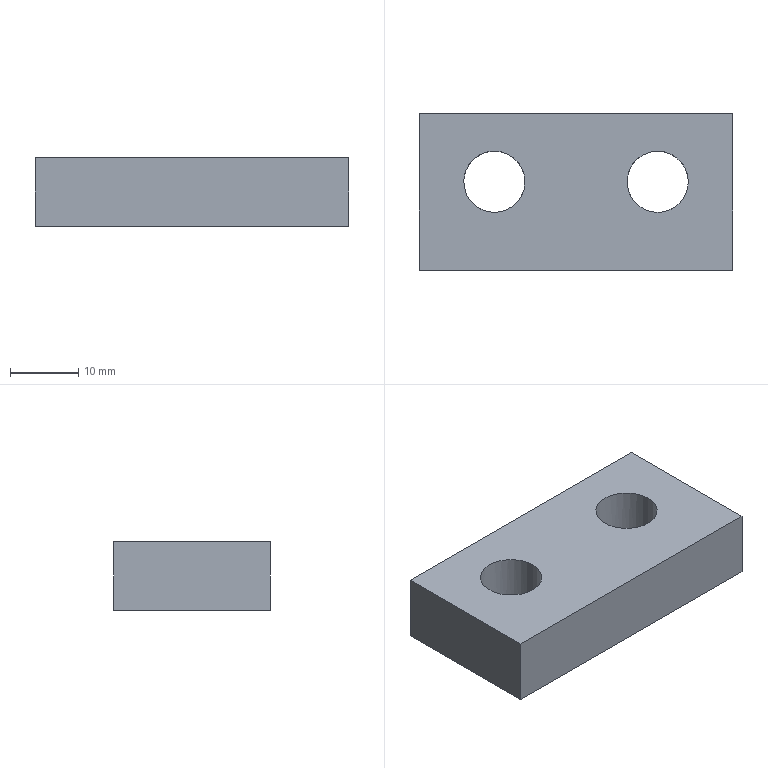Part | STEP file | gslz 2016.10.28-13_id1654_x_t | 1 solid | 8 faces | box 46 x 23 x 10 mm | volume 9308 mm3 | plane 6 | cylinder 2 | commonest cylinder face diameters 9 x2
STEP:
#1=CARTESIAN_POINT('',(0.,0.,0.));
#2=DIRECTION('',(0.,0.,1.));
#3=DIRECTION('',(1.,0.,0.));
#4=AXIS2_PLACEMENT_3D('',#1,#2,#3);
#5=CARTESIAN_POINT('',(1212.,264.496,-32.));
#6=VERTEX_POINT('',#5);
#7=CARTESIAN_POINT('',(1216.5,259.996,-32.));
#8=VERTEX_POINT('',#7);
#9=CARTESIAN_POINT('',(1212.,259.996,-32.));
#10=DIRECTION('',(0.,0.,1.));
#11=DIRECTION('',(0.,1.,0.));
#12=AXIS2_PLACEMENT_3D('',#9,#10,#11);
#13=CIRCLE('',#12,4.5);
#14=CARTESIAN_POINT('',(1365.155,250.875,-32.));
#15=DIRECTION('',(0.,0.,-1.));
#16=DIRECTION('',(-1.,0.,0.));
#17=AXIS2_PLACEMENT_3D('',#14,#15,#16);
#18=PLANE('',#17);
#19=CARTESIAN_POINT('',(153.155,13.621));
#20=CARTESIAN_POINT('',(160.949,13.621));
#21=CARTESIAN_POINT('',(157.052,6.871));
#22=CARTESIAN_POINT('',(153.155,0.121));
#23=CARTESIAN_POINT('',(149.258,6.871));
#24=CARTESIAN_POINT('',(145.361,13.621));
#25=CARTESIAN_POINT('',(153.155,13.621));
#26=(BOUNDED_CURVE()B_SPLINE_CURVE(2,(#19,#20,#21,#22,#23,#24,#25),.UNSPECIFIED.,.T.,.F.)B_SPLINE_CURVE_WITH_KNOTS((1,2,2,2,2,1),(-2.094,0.,2.094,4.189,6.283,8.378),.UNSPECIFIED.)CURVE()GEOMETRIC_REPRESENTATION_ITEM()RATIONAL_B_SPLINE_CURVE((1.,0.5,1.,0.5,1.,0.5,1.))REPRESENTATION_ITEM(''));
#27=(GEOMETRIC_REPRESENTATION_CONTEXT(2)PARAMETRIC_REPRESENTATION_CONTEXT()REPRESENTATION_CONTEXT('',''));
#28=DEFINITIONAL_REPRESENTATION('',(#26),#27);
#29=PCURVE('',#18,#28);
#30=CARTESIAN_POINT('',(1212.,259.996,-56.));
#31=DIRECTION('',(0.,0.,1.));
#32=DIRECTION('',(1.,0.,0.));
#33=AXIS2_PLACEMENT_3D('',#30,#31,#32);
#34=CYLINDRICAL_SURFACE('',#33,4.5);
#35=CARTESIAN_POINT('',(1.571,24.));
#36=DIRECTION('',(1.,0.));
#37=VECTOR('',#36,1.);
#38=LINE('',#35,#37);
#39=(GEOMETRIC_REPRESENTATION_CONTEXT(2)PARAMETRIC_REPRESENTATION_CONTEXT()REPRESENTATION_CONTEXT('',''));
#40=DEFINITIONAL_REPRESENTATION('',(#38),#39);
#41=PCURVE('',#34,#40);
#42=SURFACE_CURVE('',#13,(#29,#41),.PCURVE_S1.);
#43=EDGE_CURVE('',#6,#8,#42,.T.);
#44=ORIENTED_EDGE('',*,*,#43,.F.);
#45=CARTESIAN_POINT('',(1212.,259.996,-32.));
#46=DIRECTION('',(0.,0.,1.));
#47=DIRECTION('',(0.,1.,0.));
#48=AXIS2_PLACEMENT_3D('',#45,#46,#47);
#49=CIRCLE('',#48,4.5);
#50=CARTESIAN_POINT('',(153.155,13.621));
#51=CARTESIAN_POINT('',(160.949,13.621));
#52=CARTESIAN_POINT('',(157.052,6.871));
#53=CARTESIAN_POINT('',(153.155,0.121));
#54=CARTESIAN_POINT('',(149.258,6.871));
#55=CARTESIAN_POINT('',(145.361,13.621));
#56=CARTESIAN_POINT('',(153.155,13.621));
#57=(BOUNDED_CURVE()B_SPLINE_CURVE(2,(#50,#51,#52,#53,#54,#55,#56),.UNSPECIFIED.,.T.,.F.)B_SPLINE_CURVE_WITH_KNOTS((1,2,2,2,2,1),(-2.094,0.,2.094,4.189,6.283,8.378),.UNSPECIFIED.)CURVE()GEOMETRIC_REPRESENTATION_ITEM()RATIONAL_B_SPLINE_CURVE((1.,0.5,1.,0.5,1.,0.5,1.))REPRESENTATION_ITEM(''));
#58=(GEOMETRIC_REPRESENTATION_CONTEXT(2)PARAMETRIC_REPRESENTATION_CONTEXT()REPRESENTATION_CONTEXT('',''));
#59=DEFINITIONAL_REPRESENTATION('',(#57),#58);
#60=PCURVE('',#18,#59);
#61=CARTESIAN_POINT('',(-4.712,24.));
#62=DIRECTION('',(1.,0.));
#63=VECTOR('',#62,1.);
#64=LINE('',#61,#63);
#65=(GEOMETRIC_REPRESENTATION_CONTEXT(2)PARAMETRIC_REPRESENTATION_CONTEXT()REPRESENTATION_CONTEXT('',''));
#66=DEFINITIONAL_REPRESENTATION('',(#64),#65);
#67=PCURVE('',#34,#66);
#68=SURFACE_CURVE('',#49,(#60,#67),.PCURVE_S1.);
#69=EDGE_CURVE('',#8,#6,#68,.T.);
#70=ORIENTED_EDGE('',*,*,#69,.F.);
#71=EDGE_LOOP('',(#44,#70));
#72=FACE_BOUND('',#71,.T.);
#73=CARTESIAN_POINT('',(1236.,264.496,-32.));
#74=VERTEX_POINT('',#73);
#75=CARTESIAN_POINT('',(1240.5,259.996,-32.));
#76=VERTEX_POINT('',#75);
#77=CARTESIAN_POINT('',(1236.,259.996,-32.));
#78=DIRECTION('',(0.,0.,1.));
#79=DIRECTION('',(0.,1.,0.));
#80=AXIS2_PLACEMENT_3D('',#77,#78,#79);
#81=CIRCLE('',#80,4.5);
#82=CARTESIAN_POINT('',(129.155,13.621));
#83=CARTESIAN_POINT('',(136.949,13.621));
#84=CARTESIAN_POINT('',(133.052,6.871));
#85=CARTESIAN_POINT('',(129.155,0.121));
#86=CARTESIAN_POINT('',(125.258,6.871));
#87=CARTESIAN_POINT('',(121.361,13.621));
#88=CARTESIAN_POINT('',(129.155,13.621));
#89=(BOUNDED_CURVE()B_SPLINE_CURVE(2,(#82,#83,#84,#85,#86,#87,#88),.UNSPECIFIED.,.T.,.F.)B_SPLINE_CURVE_WITH_KNOTS((1,2,2,2,2,1),(-2.094,0.,2.094,4.189,6.283,8.378),.UNSPECIFIED.)CURVE()GEOMETRIC_REPRESENTATION_ITEM()RATIONAL_B_SPLINE_CURVE((1.,0.5,1.,0.5,1.,0.5,1.))REPRESENTATION_ITEM(''));
#90=(GEOMETRIC_REPRESENTATION_CONTEXT(2)PARAMETRIC_REPRESENTATION_CONTEXT()REPRESENTATION_CONTEXT('',''));
#91=DEFINITIONAL_REPRESENTATION('',(#89),#90);
#92=PCURVE('',#18,#91);
#93=CARTESIAN_POINT('',(1236.,259.996,-56.));
#94=DIRECTION('',(0.,0.,1.));
#95=DIRECTION('',(1.,0.,0.));
#96=AXIS2_PLACEMENT_3D('',#93,#94,#95);
#97=CYLINDRICAL_SURFACE('',#96,4.5);
#98=CARTESIAN_POINT('',(1.571,24.));
#99=DIRECTION('',(1.,0.));
#100=VECTOR('',#99,1.);
#101=LINE('',#98,#100);
#102=(GEOMETRIC_REPRESENTATION_CONTEXT(2)PARAMETRIC_REPRESENTATION_CONTEXT()REPRESENTATION_CONTEXT('',''));
#103=DEFINITIONAL_REPRESENTATION('',(#101),#102);
#104=PCURVE('',#97,#103);
#105=SURFACE_CURVE('',#81,(#92,#104),.PCURVE_S1.);
#106=EDGE_CURVE('',#74,#76,#105,.T.);
#107=ORIENTED_EDGE('',*,*,#106,.F.);
#108=CARTESIAN_POINT('',(1236.,259.996,-32.));
#109=DIRECTION('',(0.,0.,1.));
#110=DIRECTION('',(0.,1.,0.));
#111=AXIS2_PLACEMENT_3D('',#108,#109,#110);
#112=CIRCLE('',#111,4.5);
#113=CARTESIAN_POINT('',(129.155,13.621));
#114=CARTESIAN_POINT('',(136.949,13.621));
#115=CARTESIAN_POINT('',(133.052,6.871));
#116=CARTESIAN_POINT('',(129.155,0.121));
#117=CARTESIAN_POINT('',(125.258,6.871));
#118=CARTESIAN_POINT('',(121.361,13.621));
#119=CARTESIAN_POINT('',(129.155,13.621));
#120=(BOUNDED_CURVE()B_SPLINE_CURVE(2,(#113,#114,#115,#116,#117,#118,#119),.UNSPECIFIED.,.T.,.F.)B_SPLINE_CURVE_WITH_KNOTS((1,2,2,2,2,1),(-2.094,0.,2.094,4.189,6.283,8.378),.UNSPECIFIED.)CURVE()GEOMETRIC_REPRESENTATION_ITEM()RATIONAL_B_SPLINE_CURVE((1.,0.5,1.,0.5,1.,0.5,1.))REPRESENTATION_ITEM(''));
#121=(GEOMETRIC_REPRESENTATION_CONTEXT(2)PARAMETRIC_REPRESENTATION_CONTEXT()REPRESENTATION_CONTEXT('',''));
#122=DEFINITIONAL_REPRESENTATION('',(#120),#121);
#123=PCURVE('',#18,#122);
#124=CARTESIAN_POINT('',(-4.712,24.));
#125=DIRECTION('',(1.,0.));
#126=VECTOR('',#125,1.);
#127=LINE('',#124,#126);
#128=(GEOMETRIC_REPRESENTATION_CONTEXT(2)PARAMETRIC_REPRESENTATION_CONTEXT()REPRESENTATION_CONTEXT('',''));
#129=DEFINITIONAL_REPRESENTATION('',(#127),#128);
#130=PCURVE('',#97,#129);
#131=SURFACE_CURVE('',#112,(#123,#130),.PCURVE_S1.);
#132=EDGE_CURVE('',#76,#74,#131,.T.);
#133=ORIENTED_EDGE('',*,*,#132,.F.);
#134=EDGE_LOOP('',(#107,#133));
#135=FACE_BOUND('',#134,.T.);
#136=CARTESIAN_POINT('',(1247.,246.996,-32.));
#137=VERTEX_POINT('',#136);
#138=CARTESIAN_POINT('',(1201.,246.996,-32.));
#139=VERTEX_POINT('',#138);
#140=CARTESIAN_POINT('',(1302.873,246.996,-32.));
#141=DIRECTION('',(-1.,0.,0.));
#142=VECTOR('',#141,1.);
#143=LINE('',#140,#142);
#144=CARTESIAN_POINT('',(62.282,-3.879));
#145=DIRECTION('',(1.,0.));
#146=VECTOR('',#145,1.);
#147=LINE('',#144,#146);
#148=(GEOMETRIC_REPRESENTATION_CONTEXT(2)PARAMETRIC_REPRESENTATION_CONTEXT()REPRESENTATION_CONTEXT('',''));
#149=DEFINITIONAL_REPRESENTATION('',(#147),#148);
#150=PCURVE('',#18,#149);
#151=CARTESIAN_POINT('',(1302.873,246.996,-80.));
#152=DIRECTION('',(0.,1.,0.));
#153=DIRECTION('',(0.,0.,1.));
#154=AXIS2_PLACEMENT_3D('',#151,#152,#153);
#155=PLANE('',#154);
#156=CARTESIAN_POINT('',(48.,0.));
#157=DIRECTION('',(0.,-1.));
#158=VECTOR('',#157,1.);
#159=LINE('',#156,#158);
#160=(GEOMETRIC_REPRESENTATION_CONTEXT(2)PARAMETRIC_REPRESENTATION_CONTEXT()REPRESENTATION_CONTEXT('',''));
#161=DEFINITIONAL_REPRESENTATION('',(#159),#160);
#162=PCURVE('',#155,#161);
#163=SURFACE_CURVE('',#143,(#150,#162),.PCURVE_S1.);
#164=EDGE_CURVE('',#137,#139,#163,.T.);
#165=ORIENTED_EDGE('',*,*,#164,.F.);
#166=CARTESIAN_POINT('',(1247.,269.996,-32.));
#167=VERTEX_POINT('',#166);
#168=CARTESIAN_POINT('',(1247.,206.552,-32.));
#169=DIRECTION('',(0.,-1.,0.));
#170=VECTOR('',#169,1.);
#171=LINE('',#168,#170);
#172=CARTESIAN_POINT('',(118.155,-44.323));
#173=DIRECTION('',(0.,-1.));
#174=VECTOR('',#173,1.);
#175=LINE('',#172,#174);
#176=(GEOMETRIC_REPRESENTATION_CONTEXT(2)PARAMETRIC_REPRESENTATION_CONTEXT()REPRESENTATION_CONTEXT('',''));
#177=DEFINITIONAL_REPRESENTATION('',(#175),#176);
#178=PCURVE('',#18,#177);
#179=CARTESIAN_POINT('',(1247.,206.552,-56.));
#180=DIRECTION('',(1.,0.,0.));
#181=DIRECTION('',(0.,0.,-1.));
#182=AXIS2_PLACEMENT_3D('',#179,#180,#181);
#183=PLANE('',#182);
#184=CARTESIAN_POINT('',(-24.,0.));
#185=DIRECTION('',(0.,-1.));
#186=VECTOR('',#185,1.);
#187=LINE('',#184,#186);
#188=(GEOMETRIC_REPRESENTATION_CONTEXT(2)PARAMETRIC_REPRESENTATION_CONTEXT()REPRESENTATION_CONTEXT('',''));
#189=DEFINITIONAL_REPRESENTATION('',(#187),#188);
#190=PCURVE('',#183,#189);
#191=SURFACE_CURVE('',#171,(#178,#190),.PCURVE_S1.);
#192=EDGE_CURVE('',#167,#137,#191,.T.);
#193=ORIENTED_EDGE('',*,*,#192,.F.);
#194=CARTESIAN_POINT('',(1201.,269.996,-32.));
#195=VERTEX_POINT('',#194);
#196=CARTESIAN_POINT('',(1302.873,269.996,-32.));
#197=DIRECTION('',(1.,0.,0.));
#198=VECTOR('',#197,1.);
#199=LINE('',#196,#198);
#200=CARTESIAN_POINT('',(62.282,19.121));
#201=DIRECTION('',(-1.,0.));
#202=VECTOR('',#201,1.);
#203=LINE('',#200,#202);
#204=(GEOMETRIC_REPRESENTATION_CONTEXT(2)PARAMETRIC_REPRESENTATION_CONTEXT()REPRESENTATION_CONTEXT('',''));
#205=DEFINITIONAL_REPRESENTATION('',(#203),#204);
#206=PCURVE('',#18,#205);
#207=CARTESIAN_POINT('',(1302.873,269.996,-80.));
#208=DIRECTION('',(0.,1.,0.));
#209=DIRECTION('',(0.,0.,1.));
#210=AXIS2_PLACEMENT_3D('',#207,#208,#209);
#211=PLANE('',#210);
#212=CARTESIAN_POINT('',(48.,0.));
#213=DIRECTION('',(0.,1.));
#214=VECTOR('',#213,1.);
#215=LINE('',#212,#214);
#216=(GEOMETRIC_REPRESENTATION_CONTEXT(2)PARAMETRIC_REPRESENTATION_CONTEXT()REPRESENTATION_CONTEXT('',''));
#217=DEFINITIONAL_REPRESENTATION('',(#215),#216);
#218=PCURVE('',#211,#217);
#219=SURFACE_CURVE('',#199,(#206,#218),.PCURVE_S1.);
#220=EDGE_CURVE('',#195,#167,#219,.T.);
#221=ORIENTED_EDGE('',*,*,#220,.F.);
#222=CARTESIAN_POINT('',(1201.,257.5,-32.));
#223=DIRECTION('',(0.,1.,0.));
#224=VECTOR('',#223,1.);
#225=LINE('',#222,#224);
#226=CARTESIAN_POINT('',(164.155,6.625));
#227=DIRECTION('',(0.,1.));
#228=VECTOR('',#227,1.);
#229=LINE('',#226,#228);
#230=(GEOMETRIC_REPRESENTATION_CONTEXT(2)PARAMETRIC_REPRESENTATION_CONTEXT()REPRESENTATION_CONTEXT('',''));
#231=DEFINITIONAL_REPRESENTATION('',(#229),#230);
#232=PCURVE('',#18,#231);
#233=CARTESIAN_POINT('',(1201.,257.5,-37.));
#234=DIRECTION('',(-1.,0.,0.));
#235=DIRECTION('',(0.,0.,1.));
#236=AXIS2_PLACEMENT_3D('',#233,#234,#235);
#237=PLANE('',#236);
#238=CARTESIAN_POINT('',(5.,0.));
#239=DIRECTION('',(0.,1.));
#240=VECTOR('',#239,1.);
#241=LINE('',#238,#240);
#242=(GEOMETRIC_REPRESENTATION_CONTEXT(2)PARAMETRIC_REPRESENTATION_CONTEXT()REPRESENTATION_CONTEXT('',''));
#243=DEFINITIONAL_REPRESENTATION('',(#241),#242);
#244=PCURVE('',#237,#243);
#245=SURFACE_CURVE('',#225,(#232,#244),.PCURVE_S1.);
#246=EDGE_CURVE('',#139,#195,#245,.T.);
#247=ORIENTED_EDGE('',*,*,#246,.F.);
#248=EDGE_LOOP('',(#165,#193,#221,#247));
#249=FACE_BOUND('',#248,.T.);
#250=ADVANCED_FACE('',(#72,#135,#249),#18,.F.);
#251=CARTESIAN_POINT('',(1247.,246.996,-42.));
#252=VERTEX_POINT('',#251);
#253=CARTESIAN_POINT('',(1201.,246.996,-42.));
#254=VERTEX_POINT('',#253);
#255=CARTESIAN_POINT('',(1302.873,246.996,-42.));
#256=DIRECTION('',(-1.,0.,0.));
#257=VECTOR('',#256,1.);
#258=LINE('',#255,#257);
#259=CARTESIAN_POINT('',(38.,0.));
#260=DIRECTION('',(0.,-1.));
#261=VECTOR('',#260,1.);
#262=LINE('',#259,#261);
#263=(GEOMETRIC_REPRESENTATION_CONTEXT(2)PARAMETRIC_REPRESENTATION_CONTEXT()REPRESENTATION_CONTEXT('',''));
#264=DEFINITIONAL_REPRESENTATION('',(#262),#263);
#265=PCURVE('',#155,#264);
#266=CARTESIAN_POINT('',(1275.,257.5,-42.));
#267=DIRECTION('',(0.,0.,1.));
#268=DIRECTION('',(1.,0.,0.));
#269=AXIS2_PLACEMENT_3D('',#266,#267,#268);
#270=PLANE('',#269);
#271=CARTESIAN_POINT('',(27.873,-10.504));
#272=DIRECTION('',(-1.,0.));
#273=VECTOR('',#272,1.);
#274=LINE('',#271,#273);
#275=(GEOMETRIC_REPRESENTATION_CONTEXT(2)PARAMETRIC_REPRESENTATION_CONTEXT()REPRESENTATION_CONTEXT('',''));
#276=DEFINITIONAL_REPRESENTATION('',(#274),#275);
#277=PCURVE('',#270,#276);
#278=SURFACE_CURVE('',#258,(#265,#277),.PCURVE_S1.);
#279=EDGE_CURVE('',#252,#254,#278,.T.);
#280=ORIENTED_EDGE('',*,*,#279,.F.);
#281=CARTESIAN_POINT('',(1247.,246.996,-56.));
#282=DIRECTION('',(0.,0.,-1.));
#283=VECTOR('',#282,1.);
#284=LINE('',#281,#283);
#285=CARTESIAN_POINT('',(24.,-55.873));
#286=DIRECTION('',(-1.,0.));
#287=VECTOR('',#286,1.);
#288=LINE('',#285,#287);
#289=(GEOMETRIC_REPRESENTATION_CONTEXT(2)PARAMETRIC_REPRESENTATION_CONTEXT()REPRESENTATION_CONTEXT('',''));
#290=DEFINITIONAL_REPRESENTATION('',(#288),#289);
#291=PCURVE('',#155,#290);
#292=CARTESIAN_POINT('',(0.,40.444));
#293=DIRECTION('',(1.,0.));
#294=VECTOR('',#293,1.);
#295=LINE('',#292,#294);
#296=(GEOMETRIC_REPRESENTATION_CONTEXT(2)PARAMETRIC_REPRESENTATION_CONTEXT()REPRESENTATION_CONTEXT('',''));
#297=DEFINITIONAL_REPRESENTATION('',(#295),#296);
#298=PCURVE('',#183,#297);
#299=SURFACE_CURVE('',#284,(#291,#298),.PCURVE_S1.);
#300=EDGE_CURVE('',#137,#252,#299,.T.);
#301=ORIENTED_EDGE('',*,*,#300,.F.);
#302=ORIENTED_EDGE('',*,*,#164,.T.);
#303=CARTESIAN_POINT('',(1201.,246.996,-80.));
#304=DIRECTION('',(0.,0.,-1.));
#305=VECTOR('',#304,1.);
#306=LINE('',#303,#305);
#307=CARTESIAN_POINT('',(0.,-101.873));
#308=DIRECTION('',(-1.,0.));
#309=VECTOR('',#308,1.);
#310=LINE('',#307,#309);
#311=(GEOMETRIC_REPRESENTATION_CONTEXT(2)PARAMETRIC_REPRESENTATION_CONTEXT()REPRESENTATION_CONTEXT('',''));
#312=DEFINITIONAL_REPRESENTATION('',(#310),#311);
#313=PCURVE('',#155,#312);
#314=CARTESIAN_POINT('',(-43.,-10.504));
#315=DIRECTION('',(-1.,0.));
#316=VECTOR('',#315,1.);
#317=LINE('',#314,#316);
#318=(GEOMETRIC_REPRESENTATION_CONTEXT(2)PARAMETRIC_REPRESENTATION_CONTEXT()REPRESENTATION_CONTEXT('',''));
#319=DEFINITIONAL_REPRESENTATION('',(#317),#318);
#320=PCURVE('',#237,#319);
#321=SURFACE_CURVE('',#306,(#313,#320),.PCURVE_S1.);
#322=EDGE_CURVE('',#139,#254,#321,.T.);
#323=ORIENTED_EDGE('',*,*,#322,.T.);
#324=EDGE_LOOP('',(#280,#301,#302,#323));
#325=FACE_BOUND('',#324,.T.);
#326=ADVANCED_FACE('',(#325),#155,.F.);
#327=CARTESIAN_POINT('',(1247.,269.996,-42.));
#328=VERTEX_POINT('',#327);
#329=CARTESIAN_POINT('',(1247.,206.552,-42.));
#330=DIRECTION('',(0.,-1.,0.));
#331=VECTOR('',#330,1.);
#332=LINE('',#329,#331);
#333=CARTESIAN_POINT('',(-14.,0.));
#334=DIRECTION('',(0.,-1.));
#335=VECTOR('',#334,1.);
#336=LINE('',#333,#335);
#337=(GEOMETRIC_REPRESENTATION_CONTEXT(2)PARAMETRIC_REPRESENTATION_CONTEXT()REPRESENTATION_CONTEXT('',''));
#338=DEFINITIONAL_REPRESENTATION('',(#336),#337);
#339=PCURVE('',#183,#338);
#340=CARTESIAN_POINT('',(-28.,-50.948));
#341=DIRECTION('',(0.,-1.));
#342=VECTOR('',#341,1.);
#343=LINE('',#340,#342);
#344=(GEOMETRIC_REPRESENTATION_CONTEXT(2)PARAMETRIC_REPRESENTATION_CONTEXT()REPRESENTATION_CONTEXT('',''));
#345=DEFINITIONAL_REPRESENTATION('',(#343),#344);
#346=PCURVE('',#270,#345);
#347=SURFACE_CURVE('',#332,(#339,#346),.PCURVE_S1.);
#348=EDGE_CURVE('',#328,#252,#347,.T.);
#349=ORIENTED_EDGE('',*,*,#348,.F.);
#350=CARTESIAN_POINT('',(1247.,269.996,-80.));
#351=DIRECTION('',(0.,0.,-1.));
#352=VECTOR('',#351,1.);
#353=LINE('',#350,#352);
#354=CARTESIAN_POINT('',(24.,63.444));
#355=DIRECTION('',(1.,0.));
#356=VECTOR('',#355,1.);
#357=LINE('',#354,#356);
#358=(GEOMETRIC_REPRESENTATION_CONTEXT(2)PARAMETRIC_REPRESENTATION_CONTEXT()REPRESENTATION_CONTEXT('',''));
#359=DEFINITIONAL_REPRESENTATION('',(#357),#358);
#360=PCURVE('',#183,#359);
#361=CARTESIAN_POINT('',(0.,-55.873));
#362=DIRECTION('',(-1.,0.));
#363=VECTOR('',#362,1.);
#364=LINE('',#361,#363);
#365=(GEOMETRIC_REPRESENTATION_CONTEXT(2)PARAMETRIC_REPRESENTATION_CONTEXT()REPRESENTATION_CONTEXT('',''));
#366=DEFINITIONAL_REPRESENTATION('',(#364),#365);
#367=PCURVE('',#211,#366);
#368=SURFACE_CURVE('',#353,(#360,#367),.PCURVE_S1.);
#369=EDGE_CURVE('',#167,#328,#368,.T.);
#370=ORIENTED_EDGE('',*,*,#369,.F.);
#371=ORIENTED_EDGE('',*,*,#192,.T.);
#372=ORIENTED_EDGE('',*,*,#300,.T.);
#373=EDGE_LOOP('',(#349,#370,#371,#372));
#374=FACE_BOUND('',#373,.T.);
#375=ADVANCED_FACE('',(#374),#183,.T.);
#376=CARTESIAN_POINT('',(1201.,269.996,-42.));
#377=VERTEX_POINT('',#376);
#378=CARTESIAN_POINT('',(1302.873,269.996,-42.));
#379=DIRECTION('',(1.,0.,0.));
#380=VECTOR('',#379,1.);
#381=LINE('',#378,#380);
#382=CARTESIAN_POINT('',(38.,0.));
#383=DIRECTION('',(0.,1.));
#384=VECTOR('',#383,1.);
#385=LINE('',#382,#384);
#386=(GEOMETRIC_REPRESENTATION_CONTEXT(2)PARAMETRIC_REPRESENTATION_CONTEXT()REPRESENTATION_CONTEXT('',''));
#387=DEFINITIONAL_REPRESENTATION('',(#385),#386);
#388=PCURVE('',#211,#387);
#389=CARTESIAN_POINT('',(27.873,12.496));
#390=DIRECTION('',(1.,0.));
#391=VECTOR('',#390,1.);
#392=LINE('',#389,#391);
#393=(GEOMETRIC_REPRESENTATION_CONTEXT(2)PARAMETRIC_REPRESENTATION_CONTEXT()REPRESENTATION_CONTEXT('',''));
#394=DEFINITIONAL_REPRESENTATION('',(#392),#393);
#395=PCURVE('',#270,#394);
#396=SURFACE_CURVE('',#381,(#388,#395),.PCURVE_S1.);
#397=EDGE_CURVE('',#377,#328,#396,.T.);
#398=ORIENTED_EDGE('',*,*,#397,.F.);
#399=CARTESIAN_POINT('',(1201.,269.996,-37.));
#400=DIRECTION('',(0.,0.,-1.));
#401=VECTOR('',#400,1.);
#402=LINE('',#399,#401);
#403=CARTESIAN_POINT('',(43.,-101.873));
#404=DIRECTION('',(-1.,0.));
#405=VECTOR('',#404,1.);
#406=LINE('',#403,#405);
#407=(GEOMETRIC_REPRESENTATION_CONTEXT(2)PARAMETRIC_REPRESENTATION_CONTEXT()REPRESENTATION_CONTEXT('',''));
#408=DEFINITIONAL_REPRESENTATION('',(#406),#407);
#409=PCURVE('',#211,#408);
#410=CARTESIAN_POINT('',(0.,12.496));
#411=DIRECTION('',(-1.,0.));
#412=VECTOR('',#411,1.);
#413=LINE('',#410,#412);
#414=(GEOMETRIC_REPRESENTATION_CONTEXT(2)PARAMETRIC_REPRESENTATION_CONTEXT()REPRESENTATION_CONTEXT('',''));
#415=DEFINITIONAL_REPRESENTATION('',(#413),#414);
#416=PCURVE('',#237,#415);
#417=SURFACE_CURVE('',#402,(#409,#416),.PCURVE_S1.);
#418=EDGE_CURVE('',#195,#377,#417,.T.);
#419=ORIENTED_EDGE('',*,*,#418,.F.);
#420=ORIENTED_EDGE('',*,*,#220,.T.);
#421=ORIENTED_EDGE('',*,*,#369,.T.);
#422=EDGE_LOOP('',(#398,#419,#420,#421));
#423=FACE_BOUND('',#422,.T.);
#424=ADVANCED_FACE('',(#423),#211,.T.);
#425=CARTESIAN_POINT('',(1201.,257.5,-42.));
#426=DIRECTION('',(0.,1.,0.));
#427=VECTOR('',#426,1.);
#428=LINE('',#425,#427);
#429=CARTESIAN_POINT('',(-5.,0.));
#430=DIRECTION('',(0.,1.));
#431=VECTOR('',#430,1.);
#432=LINE('',#429,#431);
#433=(GEOMETRIC_REPRESENTATION_CONTEXT(2)PARAMETRIC_REPRESENTATION_CONTEXT()REPRESENTATION_CONTEXT('',''));
#434=DEFINITIONAL_REPRESENTATION('',(#432),#433);
#435=PCURVE('',#237,#434);
#436=CARTESIAN_POINT('',(-74.,0.));
#437=DIRECTION('',(0.,1.));
#438=VECTOR('',#437,1.);
#439=LINE('',#436,#438);
#440=(GEOMETRIC_REPRESENTATION_CONTEXT(2)PARAMETRIC_REPRESENTATION_CONTEXT()REPRESENTATION_CONTEXT('',''));
#441=DEFINITIONAL_REPRESENTATION('',(#439),#440);
#442=PCURVE('',#270,#441);
#443=SURFACE_CURVE('',#428,(#435,#442),.PCURVE_S1.);
#444=EDGE_CURVE('',#254,#377,#443,.T.);
#445=ORIENTED_EDGE('',*,*,#444,.F.);
#446=ORIENTED_EDGE('',*,*,#322,.F.);
#447=ORIENTED_EDGE('',*,*,#246,.T.);
#448=ORIENTED_EDGE('',*,*,#418,.T.);
#449=EDGE_LOOP('',(#445,#446,#447,#448));
#450=FACE_BOUND('',#449,.T.);
#451=ADVANCED_FACE('',(#450),#237,.T.);
#452=CARTESIAN_POINT('',(1216.5,259.996,-42.));
#453=VERTEX_POINT('',#452);
#454=CARTESIAN_POINT('',(1212.,259.996,-42.));
#455=DIRECTION('',(0.,0.,1.));
#456=DIRECTION('',(1.,0.,0.));
#457=AXIS2_PLACEMENT_3D('',#454,#455,#456);
#458=CIRCLE('',#457,4.5);
#459=CARTESIAN_POINT('',(-63.,2.496));
#460=DIRECTION('',(1.,0.));
#461=AXIS2_PLACEMENT_2D('',#459,#460);
#462=CIRCLE('',#461,4.5);
#463=(GEOMETRIC_REPRESENTATION_CONTEXT(2)PARAMETRIC_REPRESENTATION_CONTEXT()REPRESENTATION_CONTEXT('',''));
#464=DEFINITIONAL_REPRESENTATION('',(#462),#463);
#465=PCURVE('',#270,#464);
#466=CARTESIAN_POINT('',(0.,14.));
#467=DIRECTION('',(1.,0.));
#468=VECTOR('',#467,1.);
#469=LINE('',#466,#468);
#470=(GEOMETRIC_REPRESENTATION_CONTEXT(2)PARAMETRIC_REPRESENTATION_CONTEXT()REPRESENTATION_CONTEXT('',''));
#471=DEFINITIONAL_REPRESENTATION('',(#469),#470);
#472=PCURVE('',#34,#471);
#473=SURFACE_CURVE('',#458,(#465,#472),.PCURVE_S1.);
#474=EDGE_CURVE('',#453,#453,#473,.T.);
#475=ORIENTED_EDGE('',*,*,#474,.T.);
#476=EDGE_LOOP('',(#475));
#477=FACE_BOUND('',#476,.T.);
#478=CARTESIAN_POINT('',(1240.5,259.996,-42.));
#479=VERTEX_POINT('',#478);
#480=CARTESIAN_POINT('',(1236.,259.996,-42.));
#481=DIRECTION('',(0.,0.,1.));
#482=DIRECTION('',(1.,0.,0.));
#483=AXIS2_PLACEMENT_3D('',#480,#481,#482);
#484=CIRCLE('',#483,4.5);
#485=CARTESIAN_POINT('',(-39.,2.496));
#486=DIRECTION('',(1.,0.));
#487=AXIS2_PLACEMENT_2D('',#485,#486);
#488=CIRCLE('',#487,4.5);
#489=(GEOMETRIC_REPRESENTATION_CONTEXT(2)PARAMETRIC_REPRESENTATION_CONTEXT()REPRESENTATION_CONTEXT('',''));
#490=DEFINITIONAL_REPRESENTATION('',(#488),#489);
#491=PCURVE('',#270,#490);
#492=CARTESIAN_POINT('',(0.,14.));
#493=DIRECTION('',(1.,0.));
#494=VECTOR('',#493,1.);
#495=LINE('',#492,#494);
#496=(GEOMETRIC_REPRESENTATION_CONTEXT(2)PARAMETRIC_REPRESENTATION_CONTEXT()REPRESENTATION_CONTEXT('',''));
#497=DEFINITIONAL_REPRESENTATION('',(#495),#496);
#498=PCURVE('',#97,#497);
#499=SURFACE_CURVE('',#484,(#491,#498),.PCURVE_S1.);
#500=EDGE_CURVE('',#479,#479,#499,.T.);
#501=ORIENTED_EDGE('',*,*,#500,.T.);
#502=EDGE_LOOP('',(#501));
#503=FACE_BOUND('',#502,.T.);
#504=ORIENTED_EDGE('',*,*,#279,.T.);
#505=ORIENTED_EDGE('',*,*,#444,.T.);
#506=ORIENTED_EDGE('',*,*,#397,.T.);
#507=ORIENTED_EDGE('',*,*,#348,.T.);
#508=EDGE_LOOP('',(#504,#505,#506,#507));
#509=FACE_BOUND('',#508,.T.);
#510=ADVANCED_FACE('',(#477,#503,#509),#270,.F.);
#511=ORIENTED_EDGE('',*,*,#132,.F.);
#512=CARTESIAN_POINT('',(1240.5,259.996,-42.));
#513=CARTESIAN_POINT('',(1240.5,259.996,-32.));
#514=B_SPLINE_CURVE_WITH_KNOTS('',1,(#512,#513),.UNSPECIFIED.,.F.,.F.,(2,2),(14.,24.),.PIECEWISE_BEZIER_KNOTS.);
#515=CARTESIAN_POINT('',(0.,0.));
#516=DIRECTION('',(0.,1.));
#517=VECTOR('',#516,1.);
#518=LINE('',#515,#517);
#519=(GEOMETRIC_REPRESENTATION_CONTEXT(2)PARAMETRIC_REPRESENTATION_CONTEXT()REPRESENTATION_CONTEXT('',''));
#520=DEFINITIONAL_REPRESENTATION('',(#518),#519);
#521=PCURVE('',#97,#520);
#522=CARTESIAN_POINT('',(6.283,0.));
#523=DIRECTION('',(0.,1.));
#524=VECTOR('',#523,1.);
#525=LINE('',#522,#524);
#526=(GEOMETRIC_REPRESENTATION_CONTEXT(2)PARAMETRIC_REPRESENTATION_CONTEXT()REPRESENTATION_CONTEXT('',''));
#527=DEFINITIONAL_REPRESENTATION('',(#525),#526);
#528=PCURVE('',#97,#527);
#529=SEAM_CURVE('',#514,(#521,#528),.PCURVE_S1.);
#530=EDGE_CURVE('',#479,#76,#529,.T.);
#531=ORIENTED_EDGE('',*,*,#530,.F.);
#532=ORIENTED_EDGE('',*,*,#500,.T.);
#533=ORIENTED_EDGE('',*,*,#530,.T.);
#534=ORIENTED_EDGE('',*,*,#106,.F.);
#535=EDGE_LOOP('',(#511,#531,#532,#533,#534));
#536=FACE_BOUND('',#535,.F.);
#537=ADVANCED_FACE('',(#536),#97,.F.);
#538=ORIENTED_EDGE('',*,*,#69,.F.);
#539=CARTESIAN_POINT('',(1216.5,259.996,-42.));
#540=CARTESIAN_POINT('',(1216.5,259.996,-32.));
#541=B_SPLINE_CURVE_WITH_KNOTS('',1,(#539,#540),.UNSPECIFIED.,.F.,.F.,(2,2),(14.,24.),.PIECEWISE_BEZIER_KNOTS.);
#542=CARTESIAN_POINT('',(0.,0.));
#543=DIRECTION('',(0.,1.));
#544=VECTOR('',#543,1.);
#545=LINE('',#542,#544);
#546=(GEOMETRIC_REPRESENTATION_CONTEXT(2)PARAMETRIC_REPRESENTATION_CONTEXT()REPRESENTATION_CONTEXT('',''));
#547=DEFINITIONAL_REPRESENTATION('',(#545),#546);
#548=PCURVE('',#34,#547);
#549=CARTESIAN_POINT('',(6.283,0.));
#550=DIRECTION('',(0.,1.));
#551=VECTOR('',#550,1.);
#552=LINE('',#549,#551);
#553=(GEOMETRIC_REPRESENTATION_CONTEXT(2)PARAMETRIC_REPRESENTATION_CONTEXT()REPRESENTATION_CONTEXT('',''));
#554=DEFINITIONAL_REPRESENTATION('',(#552),#553);
#555=PCURVE('',#34,#554);
#556=SEAM_CURVE('',#541,(#548,#555),.PCURVE_S1.);
#557=EDGE_CURVE('',#453,#8,#556,.T.);
#558=ORIENTED_EDGE('',*,*,#557,.F.);
#559=ORIENTED_EDGE('',*,*,#474,.T.);
#560=ORIENTED_EDGE('',*,*,#557,.T.);
#561=ORIENTED_EDGE('',*,*,#43,.F.);
#562=EDGE_LOOP('',(#538,#558,#559,#560,#561));
#563=FACE_BOUND('',#562,.F.);
#564=ADVANCED_FACE('',(#563),#34,.F.);
#565=CLOSED_SHELL('',(#250,#326,#375,#424,#451,#510,#537,#564));
#566=MANIFOLD_SOLID_BREP('',#565);
#567=(LENGTH_UNIT()NAMED_UNIT(*)SI_UNIT(.MILLI.,.METRE.));
#568=UNCERTAINTY_MEASURE_WITH_UNIT(LENGTH_MEASURE(0.000002),#567,'','');
#569=(NAMED_UNIT(*)PLANE_ANGLE_UNIT()SI_UNIT($,.RADIAN.));
#570=(NAMED_UNIT(*)SI_UNIT($,.STERADIAN.)SOLID_ANGLE_UNIT());
#571=(GEOMETRIC_REPRESENTATION_CONTEXT(3)GLOBAL_UNCERTAINTY_ASSIGNED_CONTEXT((#568))GLOBAL_UNIT_ASSIGNED_CONTEXT((#567,#569,#570))REPRESENTATION_CONTEXT('',''));
#572=ADVANCED_BREP_SHAPE_REPRESENTATION('',(#4,#566),#571);